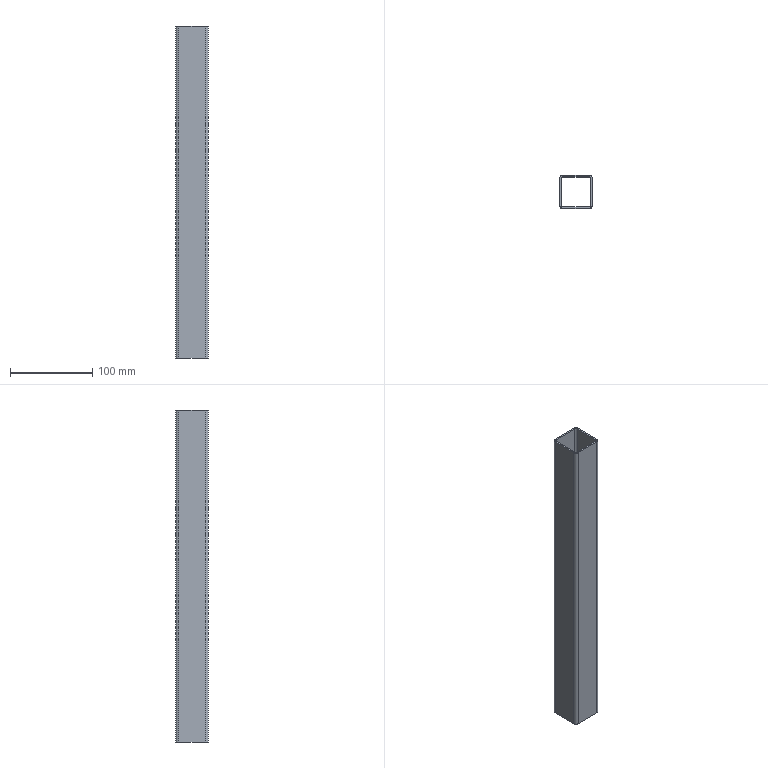Part | SolidWorks | features Fillet 2, Extrusion 1 | 1 solid | 18 faces | box 40 x 40 x 403 mm | volume 118361 mm3 | plane 10 | cylinder 8 | commonest cylinder face diameters 4 x4 8 x4
STEP:
#1=CARTESIAN_POINT('',(20.,-16.,403.));
#2=VERTEX_POINT('',#1);
#3=CARTESIAN_POINT('',(20.,16.,403.));
#4=VERTEX_POINT('',#3);
#5=CARTESIAN_POINT('',(20.,20.,403.));
#6=DIRECTION('',(0.,1.,0.));
#7=VECTOR('',#6,1000.);
#8=LINE('',#5,#7);
#9=EDGE_CURVE('',#2,#4,#8,.T.);
#10=ORIENTED_EDGE('',*,*,#9,.T.);
#11=CARTESIAN_POINT('',(16.,20.,403.));
#12=VERTEX_POINT('',#11);
#13=CARTESIAN_POINT('',(16.,16.,403.));
#14=DIRECTION('',(0.,0.,1.));
#15=DIRECTION('',(1.,0.,0.));
#16=AXIS2_PLACEMENT_3D('',#13,#14,#15);
#17=CIRCLE('',#16,4.);
#18=EDGE_CURVE('',#4,#12,#17,.T.);
#19=ORIENTED_EDGE('',*,*,#18,.T.);
#20=CARTESIAN_POINT('',(-16.,20.,403.));
#21=VERTEX_POINT('',#20);
#22=CARTESIAN_POINT('',(-20.,20.,403.));
#23=DIRECTION('',(-1.,0.,0.));
#24=VECTOR('',#23,1000.);
#25=LINE('',#22,#24);
#26=EDGE_CURVE('',#12,#21,#25,.T.);
#27=ORIENTED_EDGE('',*,*,#26,.T.);
#28=CARTESIAN_POINT('',(-20.,16.,403.));
#29=VERTEX_POINT('',#28);
#30=CARTESIAN_POINT('',(-16.,16.,403.));
#31=DIRECTION('',(0.,0.,1.));
#32=DIRECTION('',(1.,0.,0.));
#33=AXIS2_PLACEMENT_3D('',#30,#31,#32);
#34=CIRCLE('',#33,4.);
#35=EDGE_CURVE('',#21,#29,#34,.T.);
#36=ORIENTED_EDGE('',*,*,#35,.T.);
#37=CARTESIAN_POINT('',(-20.,-16.,403.));
#38=VERTEX_POINT('',#37);
#39=CARTESIAN_POINT('',(-20.,20.,403.));
#40=DIRECTION('',(0.,-1.,0.));
#41=VECTOR('',#40,1000.);
#42=LINE('',#39,#41);
#43=EDGE_CURVE('',#29,#38,#42,.T.);
#44=ORIENTED_EDGE('',*,*,#43,.T.);
#45=CARTESIAN_POINT('',(-16.,-20.,403.));
#46=VERTEX_POINT('',#45);
#47=CARTESIAN_POINT('',(-16.,-16.,403.));
#48=DIRECTION('',(0.,0.,1.));
#49=DIRECTION('',(1.,0.,0.));
#50=AXIS2_PLACEMENT_3D('',#47,#48,#49);
#51=CIRCLE('',#50,4.);
#52=EDGE_CURVE('',#38,#46,#51,.T.);
#53=ORIENTED_EDGE('',*,*,#52,.T.);
#54=CARTESIAN_POINT('',(16.,-20.,403.));
#55=VERTEX_POINT('',#54);
#56=CARTESIAN_POINT('',(-20.,-20.,403.));
#57=DIRECTION('',(1.,0.,0.));
#58=VECTOR('',#57,1000.);
#59=LINE('',#56,#58);
#60=EDGE_CURVE('',#46,#55,#59,.T.);
#61=ORIENTED_EDGE('',*,*,#60,.T.);
#62=CARTESIAN_POINT('',(16.,-16.,403.));
#63=DIRECTION('',(0.,0.,1.));
#64=DIRECTION('',(1.,0.,0.));
#65=AXIS2_PLACEMENT_3D('',#62,#63,#64);
#66=CIRCLE('',#65,4.);
#67=EDGE_CURVE('',#55,#2,#66,.T.);
#68=ORIENTED_EDGE('',*,*,#67,.T.);
#69=EDGE_LOOP('',(#10,#19,#27,#36,#44,#53,#61,#68));
#70=FACE_OUTER_BOUND('',#69,.T.);
#71=CARTESIAN_POINT('',(16.,18.,403.));
#72=VERTEX_POINT('',#71);
#73=CARTESIAN_POINT('',(-16.,18.,403.));
#74=VERTEX_POINT('',#73);
#75=CARTESIAN_POINT('',(-18.,18.,403.));
#76=DIRECTION('',(-1.,0.,0.));
#77=VECTOR('',#76,1000.);
#78=LINE('',#75,#77);
#79=EDGE_CURVE('',#72,#74,#78,.T.);
#80=ORIENTED_EDGE('',*,*,#79,.F.);
#81=CARTESIAN_POINT('',(18.,16.,403.));
#82=VERTEX_POINT('',#81);
#83=CARTESIAN_POINT('',(16.,16.,403.));
#84=DIRECTION('',(0.,0.,-1.));
#85=DIRECTION('',(1.,0.,0.));
#86=AXIS2_PLACEMENT_3D('',#83,#84,#85);
#87=CIRCLE('',#86,2.);
#88=EDGE_CURVE('',#72,#82,#87,.T.);
#89=ORIENTED_EDGE('',*,*,#88,.T.);
#90=CARTESIAN_POINT('',(18.,-16.,403.));
#91=VERTEX_POINT('',#90);
#92=CARTESIAN_POINT('',(18.,18.,403.));
#93=DIRECTION('',(0.,1.,0.));
#94=VECTOR('',#93,1000.);
#95=LINE('',#92,#94);
#96=EDGE_CURVE('',#91,#82,#95,.T.);
#97=ORIENTED_EDGE('',*,*,#96,.F.);
#98=CARTESIAN_POINT('',(16.,-18.,403.));
#99=VERTEX_POINT('',#98);
#100=CARTESIAN_POINT('',(16.,-16.,403.));
#101=DIRECTION('',(0.,0.,-1.));
#102=DIRECTION('',(1.,0.,0.));
#103=AXIS2_PLACEMENT_3D('',#100,#101,#102);
#104=CIRCLE('',#103,2.);
#105=EDGE_CURVE('',#91,#99,#104,.T.);
#106=ORIENTED_EDGE('',*,*,#105,.T.);
#107=CARTESIAN_POINT('',(-16.,-18.,403.));
#108=VERTEX_POINT('',#107);
#109=CARTESIAN_POINT('',(-18.,-18.,403.));
#110=DIRECTION('',(1.,0.,0.));
#111=VECTOR('',#110,1000.);
#112=LINE('',#109,#111);
#113=EDGE_CURVE('',#108,#99,#112,.T.);
#114=ORIENTED_EDGE('',*,*,#113,.F.);
#115=CARTESIAN_POINT('',(-18.,-16.,403.));
#116=VERTEX_POINT('',#115);
#117=CARTESIAN_POINT('',(-16.,-16.,403.));
#118=DIRECTION('',(0.,0.,-1.));
#119=DIRECTION('',(1.,0.,0.));
#120=AXIS2_PLACEMENT_3D('',#117,#118,#119);
#121=CIRCLE('',#120,2.);
#122=EDGE_CURVE('',#108,#116,#121,.T.);
#123=ORIENTED_EDGE('',*,*,#122,.T.);
#124=CARTESIAN_POINT('',(-18.,16.,403.));
#125=VERTEX_POINT('',#124);
#126=CARTESIAN_POINT('',(-18.,18.,403.));
#127=DIRECTION('',(0.,-1.,0.));
#128=VECTOR('',#127,1000.);
#129=LINE('',#126,#128);
#130=EDGE_CURVE('',#125,#116,#129,.T.);
#131=ORIENTED_EDGE('',*,*,#130,.F.);
#132=CARTESIAN_POINT('',(-16.,16.,403.));
#133=DIRECTION('',(0.,0.,-1.));
#134=DIRECTION('',(1.,0.,0.));
#135=AXIS2_PLACEMENT_3D('',#132,#133,#134);
#136=CIRCLE('',#135,2.);
#137=EDGE_CURVE('',#125,#74,#136,.T.);
#138=ORIENTED_EDGE('',*,*,#137,.T.);
#139=EDGE_LOOP('',(#80,#89,#97,#106,#114,#123,#131,#138));
#140=FACE_BOUND('',#139,.T.);
#141=CARTESIAN_POINT('',(0.,0.,403.));
#142=DIRECTION('',(0.,0.,1.));
#143=DIRECTION('',(1.,0.,0.));
#144=AXIS2_PLACEMENT_3D('',#141,#142,#143);
#145=PLANE('',#144);
#146=ADVANCED_FACE('',(#70,#140),#145,.T.);
#147=CARTESIAN_POINT('',(16.,20.,0.));
#148=VERTEX_POINT('',#147);
#149=CARTESIAN_POINT('',(-16.,20.,0.));
#150=VERTEX_POINT('',#149);
#151=CARTESIAN_POINT('',(-20.,20.,0.));
#152=DIRECTION('',(-1.,0.,0.));
#153=VECTOR('',#152,1000.);
#154=LINE('',#151,#153);
#155=EDGE_CURVE('',#148,#150,#154,.T.);
#156=ORIENTED_EDGE('',*,*,#155,.F.);
#157=CARTESIAN_POINT('',(20.,16.,0.));
#158=VERTEX_POINT('',#157);
#159=CARTESIAN_POINT('',(16.,16.,0.));
#160=DIRECTION('',(0.,0.,-1.));
#161=DIRECTION('',(1.,0.,0.));
#162=AXIS2_PLACEMENT_3D('',#159,#160,#161);
#163=CIRCLE('',#162,4.);
#164=EDGE_CURVE('',#148,#158,#163,.T.);
#165=ORIENTED_EDGE('',*,*,#164,.T.);
#166=CARTESIAN_POINT('',(20.,-16.,0.));
#167=VERTEX_POINT('',#166);
#168=CARTESIAN_POINT('',(20.,20.,0.));
#169=DIRECTION('',(0.,1.,0.));
#170=VECTOR('',#169,1000.);
#171=LINE('',#168,#170);
#172=EDGE_CURVE('',#167,#158,#171,.T.);
#173=ORIENTED_EDGE('',*,*,#172,.F.);
#174=CARTESIAN_POINT('',(16.,-20.,0.));
#175=VERTEX_POINT('',#174);
#176=CARTESIAN_POINT('',(16.,-16.,0.));
#177=DIRECTION('',(0.,0.,-1.));
#178=DIRECTION('',(1.,0.,0.));
#179=AXIS2_PLACEMENT_3D('',#176,#177,#178);
#180=CIRCLE('',#179,4.);
#181=EDGE_CURVE('',#167,#175,#180,.T.);
#182=ORIENTED_EDGE('',*,*,#181,.T.);
#183=CARTESIAN_POINT('',(-16.,-20.,0.));
#184=VERTEX_POINT('',#183);
#185=CARTESIAN_POINT('',(-20.,-20.,0.));
#186=DIRECTION('',(1.,0.,0.));
#187=VECTOR('',#186,1000.);
#188=LINE('',#185,#187);
#189=EDGE_CURVE('',#184,#175,#188,.T.);
#190=ORIENTED_EDGE('',*,*,#189,.F.);
#191=CARTESIAN_POINT('',(-20.,-16.,0.));
#192=VERTEX_POINT('',#191);
#193=CARTESIAN_POINT('',(-16.,-16.,0.));
#194=DIRECTION('',(0.,0.,-1.));
#195=DIRECTION('',(1.,0.,0.));
#196=AXIS2_PLACEMENT_3D('',#193,#194,#195);
#197=CIRCLE('',#196,4.);
#198=EDGE_CURVE('',#184,#192,#197,.T.);
#199=ORIENTED_EDGE('',*,*,#198,.T.);
#200=CARTESIAN_POINT('',(-20.,16.,0.));
#201=VERTEX_POINT('',#200);
#202=CARTESIAN_POINT('',(-20.,20.,0.));
#203=DIRECTION('',(0.,-1.,0.));
#204=VECTOR('',#203,1000.);
#205=LINE('',#202,#204);
#206=EDGE_CURVE('',#201,#192,#205,.T.);
#207=ORIENTED_EDGE('',*,*,#206,.F.);
#208=CARTESIAN_POINT('',(-16.,16.,0.));
#209=DIRECTION('',(0.,0.,-1.));
#210=DIRECTION('',(1.,0.,0.));
#211=AXIS2_PLACEMENT_3D('',#208,#209,#210);
#212=CIRCLE('',#211,4.);
#213=EDGE_CURVE('',#201,#150,#212,.T.);
#214=ORIENTED_EDGE('',*,*,#213,.T.);
#215=EDGE_LOOP('',(#156,#165,#173,#182,#190,#199,#207,#214));
#216=FACE_OUTER_BOUND('',#215,.T.);
#217=CARTESIAN_POINT('',(-16.,-18.,0.));
#218=VERTEX_POINT('',#217);
#219=CARTESIAN_POINT('',(16.,-18.,0.));
#220=VERTEX_POINT('',#219);
#221=CARTESIAN_POINT('',(-18.,-18.,0.));
#222=DIRECTION('',(1.,0.,0.));
#223=VECTOR('',#222,1000.);
#224=LINE('',#221,#223);
#225=EDGE_CURVE('',#218,#220,#224,.T.);
#226=ORIENTED_EDGE('',*,*,#225,.T.);
#227=CARTESIAN_POINT('',(18.,-16.,0.));
#228=VERTEX_POINT('',#227);
#229=CARTESIAN_POINT('',(16.,-16.,0.));
#230=DIRECTION('',(0.,0.,1.));
#231=DIRECTION('',(1.,0.,0.));
#232=AXIS2_PLACEMENT_3D('',#229,#230,#231);
#233=CIRCLE('',#232,2.);
#234=EDGE_CURVE('',#220,#228,#233,.T.);
#235=ORIENTED_EDGE('',*,*,#234,.T.);
#236=CARTESIAN_POINT('',(18.,16.,0.));
#237=VERTEX_POINT('',#236);
#238=CARTESIAN_POINT('',(18.,18.,0.));
#239=DIRECTION('',(0.,1.,0.));
#240=VECTOR('',#239,1000.);
#241=LINE('',#238,#240);
#242=EDGE_CURVE('',#228,#237,#241,.T.);
#243=ORIENTED_EDGE('',*,*,#242,.T.);
#244=CARTESIAN_POINT('',(16.,18.,0.));
#245=VERTEX_POINT('',#244);
#246=CARTESIAN_POINT('',(16.,16.,0.));
#247=DIRECTION('',(0.,0.,1.));
#248=DIRECTION('',(1.,0.,0.));
#249=AXIS2_PLACEMENT_3D('',#246,#247,#248);
#250=CIRCLE('',#249,2.);
#251=EDGE_CURVE('',#237,#245,#250,.T.);
#252=ORIENTED_EDGE('',*,*,#251,.T.);
#253=CARTESIAN_POINT('',(-16.,18.,0.));
#254=VERTEX_POINT('',#253);
#255=CARTESIAN_POINT('',(-18.,18.,0.));
#256=DIRECTION('',(-1.,0.,0.));
#257=VECTOR('',#256,1000.);
#258=LINE('',#255,#257);
#259=EDGE_CURVE('',#245,#254,#258,.T.);
#260=ORIENTED_EDGE('',*,*,#259,.T.);
#261=CARTESIAN_POINT('',(-18.,16.,0.));
#262=VERTEX_POINT('',#261);
#263=CARTESIAN_POINT('',(-16.,16.,0.));
#264=DIRECTION('',(0.,0.,1.));
#265=DIRECTION('',(1.,0.,0.));
#266=AXIS2_PLACEMENT_3D('',#263,#264,#265);
#267=CIRCLE('',#266,2.);
#268=EDGE_CURVE('',#254,#262,#267,.T.);
#269=ORIENTED_EDGE('',*,*,#268,.T.);
#270=CARTESIAN_POINT('',(-18.,-16.,0.));
#271=VERTEX_POINT('',#270);
#272=CARTESIAN_POINT('',(-18.,18.,0.));
#273=DIRECTION('',(0.,-1.,0.));
#274=VECTOR('',#273,1000.);
#275=LINE('',#272,#274);
#276=EDGE_CURVE('',#262,#271,#275,.T.);
#277=ORIENTED_EDGE('',*,*,#276,.T.);
#278=CARTESIAN_POINT('',(-16.,-16.,0.));
#279=DIRECTION('',(0.,0.,1.));
#280=DIRECTION('',(1.,0.,0.));
#281=AXIS2_PLACEMENT_3D('',#278,#279,#280);
#282=CIRCLE('',#281,2.);
#283=EDGE_CURVE('',#271,#218,#282,.T.);
#284=ORIENTED_EDGE('',*,*,#283,.T.);
#285=EDGE_LOOP('',(#226,#235,#243,#252,#260,#269,#277,#284));
#286=FACE_BOUND('',#285,.T.);
#287=CARTESIAN_POINT('',(0.,0.,0.));
#288=DIRECTION('',(0.,0.,1.));
#289=DIRECTION('',(1.,0.,0.));
#290=AXIS2_PLACEMENT_3D('',#287,#288,#289);
#291=PLANE('',#290);
#292=ADVANCED_FACE('',(#216,#286),#291,.F.);
#293=ORIENTED_EDGE('',*,*,#172,.T.);
#294=CARTESIAN_POINT('',(20.,16.,403.));
#295=DIRECTION('',(0.,0.,1.));
#296=VECTOR('',#295,1000.);
#297=LINE('',#294,#296);
#298=EDGE_CURVE('',#158,#4,#297,.T.);
#299=ORIENTED_EDGE('',*,*,#298,.T.);
#300=ORIENTED_EDGE('',*,*,#9,.F.);
#301=CARTESIAN_POINT('',(20.,-16.,403.));
#302=DIRECTION('',(0.,0.,-1.));
#303=VECTOR('',#302,1000.);
#304=LINE('',#301,#303);
#305=EDGE_CURVE('',#2,#167,#304,.T.);
#306=ORIENTED_EDGE('',*,*,#305,.T.);
#307=EDGE_LOOP('',(#293,#299,#300,#306));
#308=FACE_OUTER_BOUND('',#307,.T.);
#309=CARTESIAN_POINT('',(20.,20.,403.));
#310=DIRECTION('',(-1.,0.,0.));
#311=DIRECTION('',(0.,0.,1.));
#312=AXIS2_PLACEMENT_3D('',#309,#310,#311);
#313=PLANE('',#312);
#314=ADVANCED_FACE('',(#308),#313,.F.);
#315=ORIENTED_EDGE('',*,*,#26,.F.);
#316=CARTESIAN_POINT('',(16.,20.,403.));
#317=DIRECTION('',(0.,0.,-1.));
#318=VECTOR('',#317,1000.);
#319=LINE('',#316,#318);
#320=EDGE_CURVE('',#12,#148,#319,.T.);
#321=ORIENTED_EDGE('',*,*,#320,.T.);
#322=ORIENTED_EDGE('',*,*,#155,.T.);
#323=CARTESIAN_POINT('',(-16.,20.,403.));
#324=DIRECTION('',(0.,0.,1.));
#325=VECTOR('',#324,1000.);
#326=LINE('',#323,#325);
#327=EDGE_CURVE('',#150,#21,#326,.T.);
#328=ORIENTED_EDGE('',*,*,#327,.T.);
#329=EDGE_LOOP('',(#315,#321,#322,#328));
#330=FACE_OUTER_BOUND('',#329,.T.);
#331=CARTESIAN_POINT('',(-20.,20.,403.));
#332=DIRECTION('',(0.,-1.,0.));
#333=DIRECTION('',(0.,0.,-1.));
#334=AXIS2_PLACEMENT_3D('',#331,#332,#333);
#335=PLANE('',#334);
#336=ADVANCED_FACE('',(#330),#335,.F.);
#337=ORIENTED_EDGE('',*,*,#43,.F.);
#338=CARTESIAN_POINT('',(-20.,16.,403.));
#339=DIRECTION('',(0.,0.,-1.));
#340=VECTOR('',#339,1000.);
#341=LINE('',#338,#340);
#342=EDGE_CURVE('',#29,#201,#341,.T.);
#343=ORIENTED_EDGE('',*,*,#342,.T.);
#344=ORIENTED_EDGE('',*,*,#206,.T.);
#345=CARTESIAN_POINT('',(-20.,-16.,403.));
#346=DIRECTION('',(0.,0.,1.));
#347=VECTOR('',#346,1000.);
#348=LINE('',#345,#347);
#349=EDGE_CURVE('',#192,#38,#348,.T.);
#350=ORIENTED_EDGE('',*,*,#349,.T.);
#351=EDGE_LOOP('',(#337,#343,#344,#350));
#352=FACE_OUTER_BOUND('',#351,.T.);
#353=CARTESIAN_POINT('',(-20.,20.,403.));
#354=DIRECTION('',(1.,0.,0.));
#355=DIRECTION('',(0.,0.,-1.));
#356=AXIS2_PLACEMENT_3D('',#353,#354,#355);
#357=PLANE('',#356);
#358=ADVANCED_FACE('',(#352),#357,.F.);
#359=ORIENTED_EDGE('',*,*,#189,.T.);
#360=CARTESIAN_POINT('',(16.,-20.,403.));
#361=DIRECTION('',(0.,0.,1.));
#362=VECTOR('',#361,1000.);
#363=LINE('',#360,#362);
#364=EDGE_CURVE('',#175,#55,#363,.T.);
#365=ORIENTED_EDGE('',*,*,#364,.T.);
#366=ORIENTED_EDGE('',*,*,#60,.F.);
#367=CARTESIAN_POINT('',(-16.,-20.,403.));
#368=DIRECTION('',(0.,0.,-1.));
#369=VECTOR('',#368,1000.);
#370=LINE('',#367,#369);
#371=EDGE_CURVE('',#46,#184,#370,.T.);
#372=ORIENTED_EDGE('',*,*,#371,.T.);
#373=EDGE_LOOP('',(#359,#365,#366,#372));
#374=FACE_OUTER_BOUND('',#373,.T.);
#375=CARTESIAN_POINT('',(-20.,-20.,403.));
#376=DIRECTION('',(0.,1.,0.));
#377=DIRECTION('',(0.,0.,1.));
#378=AXIS2_PLACEMENT_3D('',#375,#376,#377);
#379=PLANE('',#378);
#380=ADVANCED_FACE('',(#374),#379,.F.);
#381=ORIENTED_EDGE('',*,*,#96,.T.);
#382=CARTESIAN_POINT('',(18.,16.,0.));
#383=DIRECTION('',(0.,0.,-1.));
#384=VECTOR('',#383,1000.);
#385=LINE('',#382,#384);
#386=EDGE_CURVE('',#82,#237,#385,.T.);
#387=ORIENTED_EDGE('',*,*,#386,.T.);
#388=ORIENTED_EDGE('',*,*,#242,.F.);
#389=CARTESIAN_POINT('',(18.,-16.,403.));
#390=DIRECTION('',(0.,0.,1.));
#391=VECTOR('',#390,1000.);
#392=LINE('',#389,#391);
#393=EDGE_CURVE('',#228,#91,#392,.T.);
#394=ORIENTED_EDGE('',*,*,#393,.T.);
#395=EDGE_LOOP('',(#381,#387,#388,#394));
#396=FACE_OUTER_BOUND('',#395,.T.);
#397=CARTESIAN_POINT('',(18.,18.,403.));
#398=DIRECTION('',(-1.,0.,0.));
#399=DIRECTION('',(0.,0.,1.));
#400=AXIS2_PLACEMENT_3D('',#397,#398,#399);
#401=PLANE('',#400);
#402=ADVANCED_FACE('',(#396),#401,.T.);
#403=ORIENTED_EDGE('',*,*,#259,.F.);
#404=CARTESIAN_POINT('',(16.,18.,403.));
#405=DIRECTION('',(0.,0.,1.));
#406=VECTOR('',#405,1000.);
#407=LINE('',#404,#406);
#408=EDGE_CURVE('',#245,#72,#407,.T.);
#409=ORIENTED_EDGE('',*,*,#408,.T.);
#410=ORIENTED_EDGE('',*,*,#79,.T.);
#411=CARTESIAN_POINT('',(-16.,18.,0.));
#412=DIRECTION('',(0.,0.,-1.));
#413=VECTOR('',#412,1000.);
#414=LINE('',#411,#413);
#415=EDGE_CURVE('',#74,#254,#414,.T.);
#416=ORIENTED_EDGE('',*,*,#415,.T.);
#417=EDGE_LOOP('',(#403,#409,#410,#416));
#418=FACE_OUTER_BOUND('',#417,.T.);
#419=CARTESIAN_POINT('',(-18.,18.,403.));
#420=DIRECTION('',(0.,-1.,0.));
#421=DIRECTION('',(0.,0.,-1.));
#422=AXIS2_PLACEMENT_3D('',#419,#420,#421);
#423=PLANE('',#422);
#424=ADVANCED_FACE('',(#418),#423,.T.);
#425=ORIENTED_EDGE('',*,*,#276,.F.);
#426=CARTESIAN_POINT('',(-18.,16.,403.));
#427=DIRECTION('',(0.,0.,1.));
#428=VECTOR('',#427,1000.);
#429=LINE('',#426,#428);
#430=EDGE_CURVE('',#262,#125,#429,.T.);
#431=ORIENTED_EDGE('',*,*,#430,.T.);
#432=ORIENTED_EDGE('',*,*,#130,.T.);
#433=CARTESIAN_POINT('',(-18.,-16.,0.));
#434=DIRECTION('',(0.,0.,-1.));
#435=VECTOR('',#434,1000.);
#436=LINE('',#433,#435);
#437=EDGE_CURVE('',#116,#271,#436,.T.);
#438=ORIENTED_EDGE('',*,*,#437,.T.);
#439=EDGE_LOOP('',(#425,#431,#432,#438));
#440=FACE_OUTER_BOUND('',#439,.T.);
#441=CARTESIAN_POINT('',(-18.,18.,403.));
#442=DIRECTION('',(1.,0.,0.));
#443=DIRECTION('',(0.,0.,-1.));
#444=AXIS2_PLACEMENT_3D('',#441,#442,#443);
#445=PLANE('',#444);
#446=ADVANCED_FACE('',(#440),#445,.T.);
#447=ORIENTED_EDGE('',*,*,#225,.F.);
#448=CARTESIAN_POINT('',(-16.,-18.,403.));
#449=DIRECTION('',(0.,0.,1.));
#450=VECTOR('',#449,1000.);
#451=LINE('',#448,#450);
#452=EDGE_CURVE('',#218,#108,#451,.T.);
#453=ORIENTED_EDGE('',*,*,#452,.T.);
#454=ORIENTED_EDGE('',*,*,#113,.T.);
#455=CARTESIAN_POINT('',(16.,-18.,0.));
#456=DIRECTION('',(0.,0.,-1.));
#457=VECTOR('',#456,1000.);
#458=LINE('',#455,#457);
#459=EDGE_CURVE('',#99,#220,#458,.T.);
#460=ORIENTED_EDGE('',*,*,#459,.T.);
#461=EDGE_LOOP('',(#447,#453,#454,#460));
#462=FACE_OUTER_BOUND('',#461,.T.);
#463=CARTESIAN_POINT('',(-18.,-18.,403.));
#464=DIRECTION('',(0.,1.,0.));
#465=DIRECTION('',(0.,0.,1.));
#466=AXIS2_PLACEMENT_3D('',#463,#464,#465);
#467=PLANE('',#466);
#468=ADVANCED_FACE('',(#462),#467,.T.);
#469=ORIENTED_EDGE('',*,*,#88,.F.);
#470=ORIENTED_EDGE('',*,*,#408,.F.);
#471=ORIENTED_EDGE('',*,*,#251,.F.);
#472=ORIENTED_EDGE('',*,*,#386,.F.);
#473=EDGE_LOOP('',(#469,#470,#471,#472));
#474=FACE_OUTER_BOUND('',#473,.T.);
#475=CARTESIAN_POINT('',(16.,16.,403.));
#476=DIRECTION('',(0.,0.,1.));
#477=DIRECTION('',(1.,0.,0.));
#478=AXIS2_PLACEMENT_3D('',#475,#476,#477);
#479=CYLINDRICAL_SURFACE('',#478,2.);
#480=ADVANCED_FACE('',(#474),#479,.F.);
#481=ORIENTED_EDGE('',*,*,#137,.F.);
#482=ORIENTED_EDGE('',*,*,#430,.F.);
#483=ORIENTED_EDGE('',*,*,#268,.F.);
#484=ORIENTED_EDGE('',*,*,#415,.F.);
#485=EDGE_LOOP('',(#481,#482,#483,#484));
#486=FACE_OUTER_BOUND('',#485,.T.);
#487=CARTESIAN_POINT('',(-16.,16.,403.));
#488=DIRECTION('',(0.,0.,1.));
#489=DIRECTION('',(1.,0.,0.));
#490=AXIS2_PLACEMENT_3D('',#487,#488,#489);
#491=CYLINDRICAL_SURFACE('',#490,2.);
#492=ADVANCED_FACE('',(#486),#491,.F.);
#493=ORIENTED_EDGE('',*,*,#122,.F.);
#494=ORIENTED_EDGE('',*,*,#452,.F.);
#495=ORIENTED_EDGE('',*,*,#283,.F.);
#496=ORIENTED_EDGE('',*,*,#437,.F.);
#497=EDGE_LOOP('',(#493,#494,#495,#496));
#498=FACE_OUTER_BOUND('',#497,.T.);
#499=CARTESIAN_POINT('',(-16.,-16.,403.));
#500=DIRECTION('',(0.,0.,1.));
#501=DIRECTION('',(1.,0.,0.));
#502=AXIS2_PLACEMENT_3D('',#499,#500,#501);
#503=CYLINDRICAL_SURFACE('',#502,2.);
#504=ADVANCED_FACE('',(#498),#503,.F.);
#505=ORIENTED_EDGE('',*,*,#105,.F.);
#506=ORIENTED_EDGE('',*,*,#393,.F.);
#507=ORIENTED_EDGE('',*,*,#234,.F.);
#508=ORIENTED_EDGE('',*,*,#459,.F.);
#509=EDGE_LOOP('',(#505,#506,#507,#508));
#510=FACE_OUTER_BOUND('',#509,.T.);
#511=CARTESIAN_POINT('',(16.,-16.,403.));
#512=DIRECTION('',(0.,0.,1.));
#513=DIRECTION('',(1.,0.,0.));
#514=AXIS2_PLACEMENT_3D('',#511,#512,#513);
#515=CYLINDRICAL_SURFACE('',#514,2.);
#516=ADVANCED_FACE('',(#510),#515,.F.);
#517=ORIENTED_EDGE('',*,*,#18,.F.);
#518=ORIENTED_EDGE('',*,*,#298,.F.);
#519=ORIENTED_EDGE('',*,*,#164,.F.);
#520=ORIENTED_EDGE('',*,*,#320,.F.);
#521=EDGE_LOOP('',(#517,#518,#519,#520));
#522=FACE_OUTER_BOUND('',#521,.T.);
#523=CARTESIAN_POINT('',(16.,16.,403.));
#524=DIRECTION('',(0.,0.,-1.));
#525=DIRECTION('',(-1.,0.,0.));
#526=AXIS2_PLACEMENT_3D('',#523,#524,#525);
#527=CYLINDRICAL_SURFACE('',#526,4.);
#528=ADVANCED_FACE('',(#522),#527,.T.);
#529=ORIENTED_EDGE('',*,*,#67,.F.);
#530=ORIENTED_EDGE('',*,*,#364,.F.);
#531=ORIENTED_EDGE('',*,*,#181,.F.);
#532=ORIENTED_EDGE('',*,*,#305,.F.);
#533=EDGE_LOOP('',(#529,#530,#531,#532));
#534=FACE_OUTER_BOUND('',#533,.T.);
#535=CARTESIAN_POINT('',(16.,-16.,403.));
#536=DIRECTION('',(0.,0.,-1.));
#537=DIRECTION('',(-1.,0.,0.));
#538=AXIS2_PLACEMENT_3D('',#535,#536,#537);
#539=CYLINDRICAL_SURFACE('',#538,4.);
#540=ADVANCED_FACE('',(#534),#539,.T.);
#541=ORIENTED_EDGE('',*,*,#35,.F.);
#542=ORIENTED_EDGE('',*,*,#327,.F.);
#543=ORIENTED_EDGE('',*,*,#213,.F.);
#544=ORIENTED_EDGE('',*,*,#342,.F.);
#545=EDGE_LOOP('',(#541,#542,#543,#544));
#546=FACE_OUTER_BOUND('',#545,.T.);
#547=CARTESIAN_POINT('',(-16.,16.,403.));
#548=DIRECTION('',(0.,0.,-1.));
#549=DIRECTION('',(-1.,0.,0.));
#550=AXIS2_PLACEMENT_3D('',#547,#548,#549);
#551=CYLINDRICAL_SURFACE('',#550,4.);
#552=ADVANCED_FACE('',(#546),#551,.T.);
#553=ORIENTED_EDGE('',*,*,#52,.F.);
#554=ORIENTED_EDGE('',*,*,#349,.F.);
#555=ORIENTED_EDGE('',*,*,#198,.F.);
#556=ORIENTED_EDGE('',*,*,#371,.F.);
#557=EDGE_LOOP('',(#553,#554,#555,#556));
#558=FACE_OUTER_BOUND('',#557,.T.);
#559=CARTESIAN_POINT('',(-16.,-16.,403.));
#560=DIRECTION('',(0.,0.,-1.));
#561=DIRECTION('',(-1.,0.,0.));
#562=AXIS2_PLACEMENT_3D('',#559,#560,#561);
#563=CYLINDRICAL_SURFACE('',#562,4.);
#564=ADVANCED_FACE('',(#558),#563,.T.);
#565=CLOSED_SHELL('',(#146,#292,#314,#336,#358,#380,#402,#424,#446,#468,#480,#492,#504,#516,#528,#540,#552,#564));
#566=MANIFOLD_SOLID_BREP('',#565);
#567=CARTESIAN_POINT('',(0.,0.,0.));
#568=DIRECTION('',(0.,0.,1.));
#569=DIRECTION('',(1.,0.,0.));
#570=AXIS2_PLACEMENT_3D('',#567,#568,#569);
#571=(LENGTH_UNIT()NAMED_UNIT(*)SI_UNIT(.MILLI.,.METRE.));
#572=UNCERTAINTY_MEASURE_WITH_UNIT(LENGTH_MEASURE(0.00001),#571,'','');
#573=(NAMED_UNIT(*)PLANE_ANGLE_UNIT()SI_UNIT($,.RADIAN.));
#574=(NAMED_UNIT(*)SI_UNIT($,.STERADIAN.)SOLID_ANGLE_UNIT());
#575=(GEOMETRIC_REPRESENTATION_CONTEXT(3)GLOBAL_UNCERTAINTY_ASSIGNED_CONTEXT((#572))GLOBAL_UNIT_ASSIGNED_CONTEXT((#571,#573,#574))REPRESENTATION_CONTEXT('',''));
#576=ADVANCED_BREP_SHAPE_REPRESENTATION('',(#566,#570),#575);